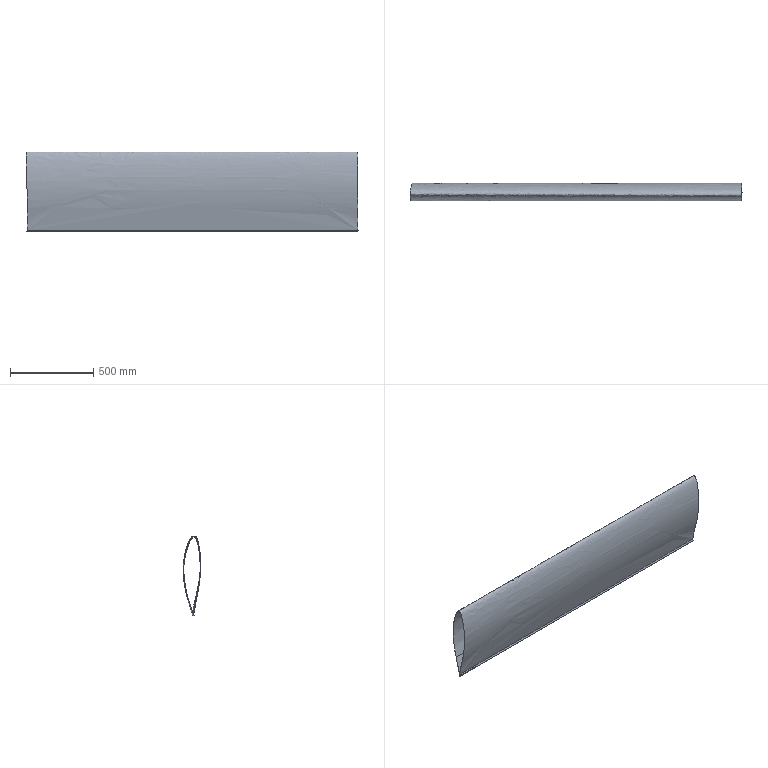Part | SolidWorks | features BaseBody 1 | 1 solid | 9 faces | box 1994 x 105.391 x 480.195 mm | volume 865818 mm3 | spline 8 | plane 1